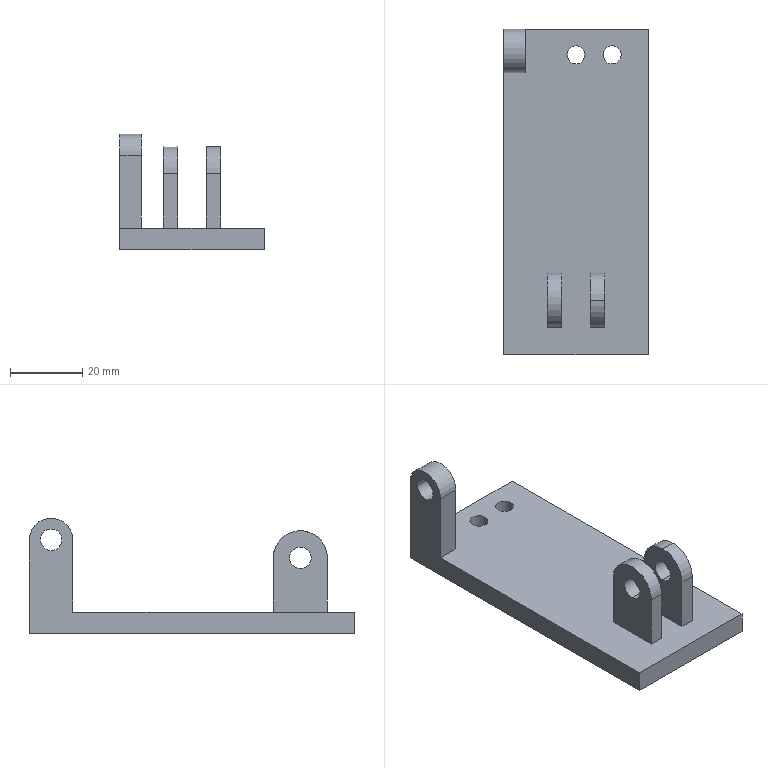Part | SolidWorks | features ICE 3, Extrusion 1, MirrorPattern 1 | 1 solid | 30 faces | box 40 x 90 x 32 mm | volume 25255 mm3 | plane 16 | cylinder 14 | commonest cylinder face diameters 6 x6 5 x4 15 x3 12 x1
STEP:
#1=CARTESIAN_POINT('',(-8.,-30.,24.));
#2=VERTEX_POINT('',#1);
#3=CARTESIAN_POINT('',(-8.,-30.,18.));
#4=VERTEX_POINT('',#3);
#5=CARTESIAN_POINT('',(-8.,-30.,21.));
#6=DIRECTION('',(1.,0.,0.));
#7=DIRECTION('',(0.,0.,-1.));
#8=AXIS2_PLACEMENT_3D('',#5,#6,#7);
#9=CIRCLE('',#8,3.);
#10=EDGE_CURVE('',#2,#4,#9,.T.);
#11=ORIENTED_EDGE('',*,*,#10,.F.);
#12=CARTESIAN_POINT('',(-4.,-30.,24.));
#13=VERTEX_POINT('',#12);
#14=CARTESIAN_POINT('',(-8.,-30.,24.));
#15=DIRECTION('',(1.,0.,0.));
#16=VECTOR('',#15,1000.);
#17=LINE('',#14,#16);
#18=EDGE_CURVE('',#2,#13,#17,.T.);
#19=ORIENTED_EDGE('',*,*,#18,.T.);
#20=CARTESIAN_POINT('',(-4.,-30.,18.));
#21=VERTEX_POINT('',#20);
#22=CARTESIAN_POINT('',(-4.,-30.,21.));
#23=DIRECTION('',(1.,0.,0.));
#24=DIRECTION('',(0.,0.,-1.));
#25=AXIS2_PLACEMENT_3D('',#22,#23,#24);
#26=CIRCLE('',#25,3.);
#27=EDGE_CURVE('',#13,#21,#26,.T.);
#28=ORIENTED_EDGE('',*,*,#27,.T.);
#29=CARTESIAN_POINT('',(-8.,-30.,18.));
#30=DIRECTION('',(1.,0.,0.));
#31=VECTOR('',#30,1000.);
#32=LINE('',#29,#31);
#33=EDGE_CURVE('',#4,#21,#32,.T.);
#34=ORIENTED_EDGE('',*,*,#33,.F.);
#35=EDGE_LOOP('',(#11,#19,#28,#34));
#36=FACE_OUTER_BOUND('',#35,.T.);
#37=CARTESIAN_POINT('',(-8.,-30.,21.));
#38=DIRECTION('',(1.,0.,0.));
#39=DIRECTION('',(0.,0.,-1.));
#40=AXIS2_PLACEMENT_3D('',#37,#38,#39);
#41=CYLINDRICAL_SURFACE('',#40,3.);
#42=ADVANCED_FACE('',(#36),#41,.F.);
#43=CARTESIAN_POINT('',(8.,-30.,24.));
#44=VERTEX_POINT('',#43);
#45=CARTESIAN_POINT('',(8.,-30.,18.));
#46=VERTEX_POINT('',#45);
#47=CARTESIAN_POINT('',(8.,-30.,21.));
#48=DIRECTION('',(1.,0.,0.));
#49=DIRECTION('',(0.,0.,-1.));
#50=AXIS2_PLACEMENT_3D('',#47,#48,#49);
#51=CIRCLE('',#50,3.);
#52=EDGE_CURVE('',#44,#46,#51,.T.);
#53=ORIENTED_EDGE('',*,*,#52,.T.);
#54=CARTESIAN_POINT('',(4.,-30.,18.));
#55=VERTEX_POINT('',#54);
#56=CARTESIAN_POINT('',(8.,-30.,18.));
#57=DIRECTION('',(-1.,0.,0.));
#58=VECTOR('',#57,1000.);
#59=LINE('',#56,#58);
#60=EDGE_CURVE('',#46,#55,#59,.T.);
#61=ORIENTED_EDGE('',*,*,#60,.T.);
#62=CARTESIAN_POINT('',(4.,-30.,24.));
#63=VERTEX_POINT('',#62);
#64=CARTESIAN_POINT('',(4.,-30.,21.));
#65=DIRECTION('',(1.,0.,0.));
#66=DIRECTION('',(0.,0.,-1.));
#67=AXIS2_PLACEMENT_3D('',#64,#65,#66);
#68=CIRCLE('',#67,3.);
#69=EDGE_CURVE('',#63,#55,#68,.T.);
#70=ORIENTED_EDGE('',*,*,#69,.F.);
#71=CARTESIAN_POINT('',(8.,-30.,24.));
#72=DIRECTION('',(-1.,0.,0.));
#73=VECTOR('',#72,1000.);
#74=LINE('',#71,#73);
#75=EDGE_CURVE('',#44,#63,#74,.T.);
#76=ORIENTED_EDGE('',*,*,#75,.F.);
#77=EDGE_LOOP('',(#53,#61,#70,#76));
#78=FACE_OUTER_BOUND('',#77,.T.);
#79=CARTESIAN_POINT('',(8.,-30.,21.));
#80=DIRECTION('',(-1.,0.,0.));
#81=DIRECTION('',(0.,0.,1.));
#82=AXIS2_PLACEMENT_3D('',#79,#80,#81);
#83=CYLINDRICAL_SURFACE('',#82,3.);
#84=ADVANCED_FACE('',(#78),#83,.F.);
#85=CARTESIAN_POINT('',(8.,-30.,28.5));
#86=VERTEX_POINT('',#85);
#87=CARTESIAN_POINT('',(8.,-37.5,21.));
#88=VERTEX_POINT('',#87);
#89=CARTESIAN_POINT('',(8.,-30.,21.));
#90=DIRECTION('',(1.,0.,0.));
#91=DIRECTION('',(0.,0.,-1.));
#92=AXIS2_PLACEMENT_3D('',#89,#90,#91);
#93=CIRCLE('',#92,7.5);
#94=EDGE_CURVE('',#86,#88,#93,.T.);
#95=ORIENTED_EDGE('',*,*,#94,.F.);
#96=CARTESIAN_POINT('',(4.,-30.,28.5));
#97=VERTEX_POINT('',#96);
#98=CARTESIAN_POINT('',(8.,-30.,28.5));
#99=DIRECTION('',(-1.,0.,0.));
#100=VECTOR('',#99,1000.);
#101=LINE('',#98,#100);
#102=EDGE_CURVE('',#86,#97,#101,.T.);
#103=ORIENTED_EDGE('',*,*,#102,.T.);
#104=CARTESIAN_POINT('',(4.,-37.5,21.));
#105=VERTEX_POINT('',#104);
#106=CARTESIAN_POINT('',(4.,-30.,21.));
#107=DIRECTION('',(1.,0.,0.));
#108=DIRECTION('',(0.,0.,-1.));
#109=AXIS2_PLACEMENT_3D('',#106,#107,#108);
#110=CIRCLE('',#109,7.5);
#111=EDGE_CURVE('',#97,#105,#110,.T.);
#112=ORIENTED_EDGE('',*,*,#111,.T.);
#113=CARTESIAN_POINT('',(8.,-37.5,21.));
#114=DIRECTION('',(-1.,0.,0.));
#115=VECTOR('',#114,1000.);
#116=LINE('',#113,#115);
#117=EDGE_CURVE('',#88,#105,#116,.T.);
#118=ORIENTED_EDGE('',*,*,#117,.F.);
#119=EDGE_LOOP('',(#95,#103,#112,#118));
#120=FACE_OUTER_BOUND('',#119,.T.);
#121=CARTESIAN_POINT('',(8.,-30.,21.));
#122=DIRECTION('',(-1.,0.,0.));
#123=DIRECTION('',(0.,0.,1.));
#124=AXIS2_PLACEMENT_3D('',#121,#122,#123);
#125=CYLINDRICAL_SURFACE('',#124,7.5);
#126=ADVANCED_FACE('',(#120),#125,.T.);
#127=CARTESIAN_POINT('',(-14.,42.,26.));
#128=VERTEX_POINT('',#127);
#129=CARTESIAN_POINT('',(-14.,36.,26.));
#130=VERTEX_POINT('',#129);
#131=CARTESIAN_POINT('',(-14.,39.,26.));
#132=DIRECTION('',(-1.,0.,0.));
#133=DIRECTION('',(0.,-1.,0.));
#134=AXIS2_PLACEMENT_3D('',#131,#132,#133);
#135=CIRCLE('',#134,3.);
#136=EDGE_CURVE('',#128,#130,#135,.T.);
#137=ORIENTED_EDGE('',*,*,#136,.F.);
#138=CARTESIAN_POINT('',(-20.,42.,26.));
#139=VERTEX_POINT('',#138);
#140=CARTESIAN_POINT('',(-14.,42.,26.));
#141=DIRECTION('',(-1.,0.,0.));
#142=VECTOR('',#141,1000.);
#143=LINE('',#140,#142);
#144=EDGE_CURVE('',#128,#139,#143,.T.);
#145=ORIENTED_EDGE('',*,*,#144,.T.);
#146=CARTESIAN_POINT('',(-20.,36.,26.));
#147=VERTEX_POINT('',#146);
#148=CARTESIAN_POINT('',(-20.,39.,26.));
#149=DIRECTION('',(-1.,0.,0.));
#150=DIRECTION('',(0.,-1.,0.));
#151=AXIS2_PLACEMENT_3D('',#148,#149,#150);
#152=CIRCLE('',#151,3.);
#153=EDGE_CURVE('',#139,#147,#152,.T.);
#154=ORIENTED_EDGE('',*,*,#153,.T.);
#155=CARTESIAN_POINT('',(-14.,36.,26.));
#156=DIRECTION('',(-1.,0.,0.));
#157=VECTOR('',#156,1000.);
#158=LINE('',#155,#157);
#159=EDGE_CURVE('',#130,#147,#158,.T.);
#160=ORIENTED_EDGE('',*,*,#159,.F.);
#161=EDGE_LOOP('',(#137,#145,#154,#160));
#162=FACE_OUTER_BOUND('',#161,.T.);
#163=CARTESIAN_POINT('',(-14.,39.,26.));
#164=DIRECTION('',(-1.,0.,0.));
#165=DIRECTION('',(0.,-1.,0.));
#166=AXIS2_PLACEMENT_3D('',#163,#164,#165);
#167=CYLINDRICAL_SURFACE('',#166,3.);
#168=ADVANCED_FACE('',(#162),#167,.F.);
#169=CARTESIAN_POINT('',(-2.5,38.,0.));
#170=VERTEX_POINT('',#169);
#171=CARTESIAN_POINT('',(2.5,38.,0.));
#172=VERTEX_POINT('',#171);
#173=CARTESIAN_POINT('',(0.,38.,0.));
#174=DIRECTION('',(0.,0.,1.));
#175=DIRECTION('',(1.,0.,0.));
#176=AXIS2_PLACEMENT_3D('',#173,#174,#175);
#177=CIRCLE('',#176,2.5);
#178=EDGE_CURVE('',#170,#172,#177,.T.);
#179=ORIENTED_EDGE('',*,*,#178,.F.);
#180=CARTESIAN_POINT('',(-2.5,38.,6.));
#181=VERTEX_POINT('',#180);
#182=CARTESIAN_POINT('',(-2.5,38.,0.));
#183=DIRECTION('',(0.,0.,1.));
#184=VECTOR('',#183,1000.);
#185=LINE('',#182,#184);
#186=EDGE_CURVE('',#170,#181,#185,.T.);
#187=ORIENTED_EDGE('',*,*,#186,.T.);
#188=CARTESIAN_POINT('',(2.5,38.,6.));
#189=VERTEX_POINT('',#188);
#190=CARTESIAN_POINT('',(0.,38.,6.));
#191=DIRECTION('',(0.,0.,1.));
#192=DIRECTION('',(1.,0.,0.));
#193=AXIS2_PLACEMENT_3D('',#190,#191,#192);
#194=CIRCLE('',#193,2.5);
#195=EDGE_CURVE('',#181,#189,#194,.T.);
#196=ORIENTED_EDGE('',*,*,#195,.T.);
#197=CARTESIAN_POINT('',(2.5,38.,0.));
#198=DIRECTION('',(0.,0.,1.));
#199=VECTOR('',#198,1000.);
#200=LINE('',#197,#199);
#201=EDGE_CURVE('',#172,#189,#200,.T.);
#202=ORIENTED_EDGE('',*,*,#201,.F.);
#203=EDGE_LOOP('',(#179,#187,#196,#202));
#204=FACE_OUTER_BOUND('',#203,.T.);
#205=CARTESIAN_POINT('',(0.,38.,0.));
#206=DIRECTION('',(0.,0.,1.));
#207=DIRECTION('',(1.,0.,0.));
#208=AXIS2_PLACEMENT_3D('',#205,#206,#207);
#209=CYLINDRICAL_SURFACE('',#208,2.5);
#210=ADVANCED_FACE('',(#204),#209,.F.);
#211=CARTESIAN_POINT('',(7.5,38.,0.));
#212=VERTEX_POINT('',#211);
#213=CARTESIAN_POINT('',(12.5,38.,0.));
#214=VERTEX_POINT('',#213);
#215=CARTESIAN_POINT('',(10.,38.,0.));
#216=DIRECTION('',(0.,0.,1.));
#217=DIRECTION('',(1.,0.,0.));
#218=AXIS2_PLACEMENT_3D('',#215,#216,#217);
#219=CIRCLE('',#218,2.5);
#220=EDGE_CURVE('',#212,#214,#219,.T.);
#221=ORIENTED_EDGE('',*,*,#220,.F.);
#222=CARTESIAN_POINT('',(7.5,38.,6.));
#223=VERTEX_POINT('',#222);
#224=CARTESIAN_POINT('',(7.5,38.,0.));
#225=DIRECTION('',(0.,0.,1.));
#226=VECTOR('',#225,1000.);
#227=LINE('',#224,#226);
#228=EDGE_CURVE('',#212,#223,#227,.T.);
#229=ORIENTED_EDGE('',*,*,#228,.T.);
#230=CARTESIAN_POINT('',(12.5,38.,6.));
#231=VERTEX_POINT('',#230);
#232=CARTESIAN_POINT('',(10.,38.,6.));
#233=DIRECTION('',(0.,0.,1.));
#234=DIRECTION('',(1.,0.,0.));
#235=AXIS2_PLACEMENT_3D('',#232,#233,#234);
#236=CIRCLE('',#235,2.5);
#237=EDGE_CURVE('',#223,#231,#236,.T.);
#238=ORIENTED_EDGE('',*,*,#237,.T.);
#239=CARTESIAN_POINT('',(12.5,38.,0.));
#240=DIRECTION('',(0.,0.,1.));
#241=VECTOR('',#240,1000.);
#242=LINE('',#239,#241);
#243=EDGE_CURVE('',#214,#231,#242,.T.);
#244=ORIENTED_EDGE('',*,*,#243,.F.);
#245=EDGE_LOOP('',(#221,#229,#238,#244));
#246=FACE_OUTER_BOUND('',#245,.T.);
#247=CARTESIAN_POINT('',(10.,38.,0.));
#248=DIRECTION('',(0.,0.,1.));
#249=DIRECTION('',(1.,0.,0.));
#250=AXIS2_PLACEMENT_3D('',#247,#248,#249);
#251=CYLINDRICAL_SURFACE('',#250,2.5);
#252=ADVANCED_FACE('',(#246),#251,.F.);
#253=CARTESIAN_POINT('',(-8.,-37.5,6.));
#254=VERTEX_POINT('',#253);
#255=CARTESIAN_POINT('',(-8.,-22.5,6.));
#256=VERTEX_POINT('',#255);
#257=CARTESIAN_POINT('',(-8.,-22.5,6.));
#258=DIRECTION('',(0.,1.,0.));
#259=VECTOR('',#258,1000.);
#260=LINE('',#257,#259);
#261=EDGE_CURVE('',#254,#256,#260,.T.);
#262=ORIENTED_EDGE('',*,*,#261,.T.);
#263=CARTESIAN_POINT('',(-4.,-22.5,6.));
#264=VERTEX_POINT('',#263);
#265=CARTESIAN_POINT('',(-8.,-22.5,6.));
#266=DIRECTION('',(1.,0.,0.));
#267=VECTOR('',#266,1000.);
#268=LINE('',#265,#267);
#269=EDGE_CURVE('',#256,#264,#268,.T.);
#270=ORIENTED_EDGE('',*,*,#269,.T.);
#271=CARTESIAN_POINT('',(-4.,-37.5,6.));
#272=VERTEX_POINT('',#271);
#273=CARTESIAN_POINT('',(-4.,-22.5,6.));
#274=DIRECTION('',(0.,1.,0.));
#275=VECTOR('',#274,1000.);
#276=LINE('',#273,#275);
#277=EDGE_CURVE('',#272,#264,#276,.T.);
#278=ORIENTED_EDGE('',*,*,#277,.F.);
#279=CARTESIAN_POINT('',(-8.,-37.5,6.));
#280=DIRECTION('',(1.,0.,0.));
#281=VECTOR('',#280,1000.);
#282=LINE('',#279,#281);
#283=EDGE_CURVE('',#254,#272,#282,.T.);
#284=ORIENTED_EDGE('',*,*,#283,.F.);
#285=EDGE_LOOP('',(#262,#270,#278,#284));
#286=FACE_BOUND('',#285,.T.);
#287=CARTESIAN_POINT('',(0.,38.,6.));
#288=DIRECTION('',(0.,0.,1.));
#289=DIRECTION('',(1.,0.,0.));
#290=AXIS2_PLACEMENT_3D('',#287,#288,#289);
#291=CIRCLE('',#290,2.5);
#292=EDGE_CURVE('',#189,#181,#291,.T.);
#293=ORIENTED_EDGE('',*,*,#292,.F.);
#294=ORIENTED_EDGE('',*,*,#195,.F.);
#295=EDGE_LOOP('',(#293,#294));
#296=FACE_BOUND('',#295,.T.);
#297=CARTESIAN_POINT('',(10.,38.,6.));
#298=DIRECTION('',(0.,0.,1.));
#299=DIRECTION('',(1.,0.,0.));
#300=AXIS2_PLACEMENT_3D('',#297,#298,#299);
#301=CIRCLE('',#300,2.5);
#302=EDGE_CURVE('',#231,#223,#301,.T.);
#303=ORIENTED_EDGE('',*,*,#302,.F.);
#304=ORIENTED_EDGE('',*,*,#237,.F.);
#305=EDGE_LOOP('',(#303,#304));
#306=FACE_BOUND('',#305,.T.);
#307=CARTESIAN_POINT('',(20.,45.,6.));
#308=VERTEX_POINT('',#307);
#309=CARTESIAN_POINT('',(-14.,45.,6.));
#310=VERTEX_POINT('',#309);
#311=CARTESIAN_POINT('',(-20.,45.,6.));
#312=DIRECTION('',(-1.,0.,0.));
#313=VECTOR('',#312,1000.);
#314=LINE('',#311,#313);
#315=EDGE_CURVE('',#308,#310,#314,.T.);
#316=ORIENTED_EDGE('',*,*,#315,.T.);
#317=CARTESIAN_POINT('',(-14.,33.,6.));
#318=VERTEX_POINT('',#317);
#319=CARTESIAN_POINT('',(-14.,45.,6.));
#320=DIRECTION('',(0.,-1.,0.));
#321=VECTOR('',#320,1000.);
#322=LINE('',#319,#321);
#323=EDGE_CURVE('',#310,#318,#322,.T.);
#324=ORIENTED_EDGE('',*,*,#323,.T.);
#325=CARTESIAN_POINT('',(-20.,33.,6.));
#326=VERTEX_POINT('',#325);
#327=CARTESIAN_POINT('',(-14.,33.,6.));
#328=DIRECTION('',(-1.,0.,0.));
#329=VECTOR('',#328,1000.);
#330=LINE('',#327,#329);
#331=EDGE_CURVE('',#318,#326,#330,.T.);
#332=ORIENTED_EDGE('',*,*,#331,.T.);
#333=CARTESIAN_POINT('',(-20.,-45.,6.));
#334=VERTEX_POINT('',#333);
#335=CARTESIAN_POINT('',(-20.,45.,6.));
#336=DIRECTION('',(0.,-1.,0.));
#337=VECTOR('',#336,1000.);
#338=LINE('',#335,#337);
#339=EDGE_CURVE('',#326,#334,#338,.T.);
#340=ORIENTED_EDGE('',*,*,#339,.T.);
#341=CARTESIAN_POINT('',(20.,-45.,6.));
#342=VERTEX_POINT('',#341);
#343=CARTESIAN_POINT('',(-20.,-45.,6.));
#344=DIRECTION('',(1.,0.,0.));
#345=VECTOR('',#344,1000.);
#346=LINE('',#343,#345);
#347=EDGE_CURVE('',#334,#342,#346,.T.);
#348=ORIENTED_EDGE('',*,*,#347,.T.);
#349=CARTESIAN_POINT('',(20.,45.,6.));
#350=DIRECTION('',(0.,1.,0.));
#351=VECTOR('',#350,1000.);
#352=LINE('',#349,#351);
#353=EDGE_CURVE('',#342,#308,#352,.T.);
#354=ORIENTED_EDGE('',*,*,#353,.T.);
#355=EDGE_LOOP('',(#316,#324,#332,#340,#348,#354));
#356=FACE_OUTER_BOUND('',#355,.T.);
#357=CARTESIAN_POINT('',(8.,-37.5,6.));
#358=VERTEX_POINT('',#357);
#359=CARTESIAN_POINT('',(8.,-22.5,6.));
#360=VERTEX_POINT('',#359);
#361=CARTESIAN_POINT('',(8.,-22.5,6.));
#362=DIRECTION('',(0.,1.,0.));
#363=VECTOR('',#362,1000.);
#364=LINE('',#361,#363);
#365=EDGE_CURVE('',#358,#360,#364,.T.);
#366=ORIENTED_EDGE('',*,*,#365,.F.);
#367=CARTESIAN_POINT('',(4.,-37.5,6.));
#368=VERTEX_POINT('',#367);
#369=CARTESIAN_POINT('',(8.,-37.5,6.));
#370=DIRECTION('',(-1.,0.,0.));
#371=VECTOR('',#370,1000.);
#372=LINE('',#369,#371);
#373=EDGE_CURVE('',#358,#368,#372,.T.);
#374=ORIENTED_EDGE('',*,*,#373,.T.);
#375=CARTESIAN_POINT('',(4.,-22.5,6.));
#376=VERTEX_POINT('',#375);
#377=CARTESIAN_POINT('',(4.,-22.5,6.));
#378=DIRECTION('',(0.,1.,0.));
#379=VECTOR('',#378,1000.);
#380=LINE('',#377,#379);
#381=EDGE_CURVE('',#368,#376,#380,.T.);
#382=ORIENTED_EDGE('',*,*,#381,.T.);
#383=CARTESIAN_POINT('',(8.,-22.5,6.));
#384=DIRECTION('',(-1.,0.,0.));
#385=VECTOR('',#384,1000.);
#386=LINE('',#383,#385);
#387=EDGE_CURVE('',#360,#376,#386,.T.);
#388=ORIENTED_EDGE('',*,*,#387,.F.);
#389=EDGE_LOOP('',(#366,#374,#382,#388));
#390=FACE_BOUND('',#389,.T.);
#391=CARTESIAN_POINT('',(0.,0.,6.));
#392=DIRECTION('',(0.,0.,1.));
#393=DIRECTION('',(1.,0.,0.));
#394=AXIS2_PLACEMENT_3D('',#391,#392,#393);
#395=PLANE('',#394);
#396=ADVANCED_FACE('',(#286,#296,#306,#356,#390),#395,.T.);
#397=CARTESIAN_POINT('',(20.,-45.,0.));
#398=VERTEX_POINT('',#397);
#399=CARTESIAN_POINT('',(20.,45.,0.));
#400=VERTEX_POINT('',#399);
#401=CARTESIAN_POINT('',(20.,45.,0.));
#402=DIRECTION('',(0.,1.,0.));
#403=VECTOR('',#402,1000.);
#404=LINE('',#401,#403);
#405=EDGE_CURVE('',#398,#400,#404,.T.);
#406=ORIENTED_EDGE('',*,*,#405,.T.);
#407=CARTESIAN_POINT('',(20.,45.,6.));
#408=DIRECTION('',(0.,0.,-1.));
#409=VECTOR('',#408,1000.);
#410=LINE('',#407,#409);
#411=EDGE_CURVE('',#308,#400,#410,.T.);
#412=ORIENTED_EDGE('',*,*,#411,.F.);
#413=ORIENTED_EDGE('',*,*,#353,.F.);
#414=CARTESIAN_POINT('',(20.,-45.,6.));
#415=DIRECTION('',(0.,0.,-1.));
#416=VECTOR('',#415,1000.);
#417=LINE('',#414,#416);
#418=EDGE_CURVE('',#342,#398,#417,.T.);
#419=ORIENTED_EDGE('',*,*,#418,.T.);
#420=EDGE_LOOP('',(#406,#412,#413,#419));
#421=FACE_OUTER_BOUND('',#420,.T.);
#422=CARTESIAN_POINT('',(20.,45.,6.));
#423=DIRECTION('',(-1.,0.,0.));
#424=DIRECTION('',(0.,-1.,0.));
#425=AXIS2_PLACEMENT_3D('',#422,#423,#424);
#426=PLANE('',#425);
#427=ADVANCED_FACE('',(#421),#426,.F.);
#428=CARTESIAN_POINT('',(-20.,45.,0.));
#429=VERTEX_POINT('',#428);
#430=CARTESIAN_POINT('',(-20.,45.,0.));
#431=DIRECTION('',(-1.,0.,0.));
#432=VECTOR('',#431,1000.);
#433=LINE('',#430,#432);
#434=EDGE_CURVE('',#400,#429,#433,.T.);
#435=ORIENTED_EDGE('',*,*,#434,.T.);
#436=CARTESIAN_POINT('',(-20.,45.,26.));
#437=VERTEX_POINT('',#436);
#438=CARTESIAN_POINT('',(-20.,45.,6.));
#439=DIRECTION('',(0.,0.,-1.));
#440=VECTOR('',#439,1000.);
#441=LINE('',#438,#440);
#442=EDGE_CURVE('',#437,#429,#441,.T.);
#443=ORIENTED_EDGE('',*,*,#442,.F.);
#444=CARTESIAN_POINT('',(-14.,45.,26.));
#445=VERTEX_POINT('',#444);
#446=CARTESIAN_POINT('',(-14.,45.,26.));
#447=DIRECTION('',(-1.,0.,0.));
#448=VECTOR('',#447,1000.);
#449=LINE('',#446,#448);
#450=EDGE_CURVE('',#445,#437,#449,.T.);
#451=ORIENTED_EDGE('',*,*,#450,.F.);
#452=CARTESIAN_POINT('',(-14.,45.,26.));
#453=DIRECTION('',(0.,0.,-1.));
#454=VECTOR('',#453,1000.);
#455=LINE('',#452,#454);
#456=EDGE_CURVE('',#445,#310,#455,.T.);
#457=ORIENTED_EDGE('',*,*,#456,.T.);
#458=ORIENTED_EDGE('',*,*,#315,.F.);
#459=ORIENTED_EDGE('',*,*,#411,.T.);
#460=EDGE_LOOP('',(#435,#443,#451,#457,#458,#459));
#461=FACE_OUTER_BOUND('',#460,.T.);
#462=CARTESIAN_POINT('',(-20.,45.,6.));
#463=DIRECTION('',(0.,-1.,0.));
#464=DIRECTION('',(0.,0.,-1.));
#465=AXIS2_PLACEMENT_3D('',#462,#463,#464);
#466=PLANE('',#465);
#467=ADVANCED_FACE('',(#461),#466,.F.);
#468=CARTESIAN_POINT('',(-20.,-45.,0.));
#469=VERTEX_POINT('',#468);
#470=CARTESIAN_POINT('',(-20.,45.,0.));
#471=DIRECTION('',(0.,-1.,0.));
#472=VECTOR('',#471,1000.);
#473=LINE('',#470,#472);
#474=EDGE_CURVE('',#429,#469,#473,.T.);
#475=ORIENTED_EDGE('',*,*,#474,.T.);
#476=CARTESIAN_POINT('',(-20.,-45.,6.));
#477=DIRECTION('',(0.,0.,-1.));
#478=VECTOR('',#477,1000.);
#479=LINE('',#476,#478);
#480=EDGE_CURVE('',#334,#469,#479,.T.);
#481=ORIENTED_EDGE('',*,*,#480,.F.);
#482=ORIENTED_EDGE('',*,*,#339,.F.);
#483=CARTESIAN_POINT('',(-20.,33.,26.));
#484=VERTEX_POINT('',#483);
#485=CARTESIAN_POINT('',(-20.,33.,6.));
#486=DIRECTION('',(0.,0.,1.));
#487=VECTOR('',#486,1000.);
#488=LINE('',#485,#487);
#489=EDGE_CURVE('',#326,#484,#488,.T.);
#490=ORIENTED_EDGE('',*,*,#489,.T.);
#491=CARTESIAN_POINT('',(-20.,39.,26.));
#492=DIRECTION('',(-1.,0.,0.));
#493=DIRECTION('',(0.,-1.,0.));
#494=AXIS2_PLACEMENT_3D('',#491,#492,#493);
#495=CIRCLE('',#494,6.);
#496=EDGE_CURVE('',#484,#437,#495,.T.);
#497=ORIENTED_EDGE('',*,*,#496,.T.);
#498=ORIENTED_EDGE('',*,*,#442,.T.);
#499=EDGE_LOOP('',(#475,#481,#482,#490,#497,#498));
#500=FACE_OUTER_BOUND('',#499,.T.);
#501=CARTESIAN_POINT('',(-20.,39.,26.));
#502=DIRECTION('',(-1.,0.,0.));
#503=DIRECTION('',(0.,-1.,0.));
#504=AXIS2_PLACEMENT_3D('',#501,#502,#503);
#505=CIRCLE('',#504,3.);
#506=EDGE_CURVE('',#147,#139,#505,.T.);
#507=ORIENTED_EDGE('',*,*,#506,.F.);
#508=ORIENTED_EDGE('',*,*,#153,.F.);
#509=EDGE_LOOP('',(#507,#508));
#510=FACE_BOUND('',#509,.T.);
#511=CARTESIAN_POINT('',(-20.,45.,6.));
#512=DIRECTION('',(1.,0.,0.));
#513=DIRECTION('',(0.,1.,0.));
#514=AXIS2_PLACEMENT_3D('',#511,#512,#513);
#515=PLANE('',#514);
#516=ADVANCED_FACE('',(#500,#510),#515,.F.);
#517=CARTESIAN_POINT('',(-20.,-45.,0.));
#518=DIRECTION('',(1.,0.,0.));
#519=VECTOR('',#518,1000.);
#520=LINE('',#517,#519);
#521=EDGE_CURVE('',#469,#398,#520,.T.);
#522=ORIENTED_EDGE('',*,*,#521,.T.);
#523=ORIENTED_EDGE('',*,*,#418,.F.);
#524=ORIENTED_EDGE('',*,*,#347,.F.);
#525=ORIENTED_EDGE('',*,*,#480,.T.);
#526=EDGE_LOOP('',(#522,#523,#524,#525));
#527=FACE_OUTER_BOUND('',#526,.T.);
#528=CARTESIAN_POINT('',(-20.,-45.,6.));
#529=DIRECTION('',(0.,1.,0.));
#530=DIRECTION('',(0.,0.,1.));
#531=AXIS2_PLACEMENT_3D('',#528,#529,#530);
#532=PLANE('',#531);
#533=ADVANCED_FACE('',(#527),#532,.F.);
#534=CARTESIAN_POINT('',(0.,38.,0.));
#535=DIRECTION('',(0.,0.,1.));
#536=DIRECTION('',(1.,0.,0.));
#537=AXIS2_PLACEMENT_3D('',#534,#535,#536);
#538=CIRCLE('',#537,2.5);
#539=EDGE_CURVE('',#172,#170,#538,.T.);
#540=ORIENTED_EDGE('',*,*,#539,.T.);
#541=ORIENTED_EDGE('',*,*,#178,.T.);
#542=EDGE_LOOP('',(#540,#541));
#543=FACE_BOUND('',#542,.T.);
#544=CARTESIAN_POINT('',(10.,38.,0.));
#545=DIRECTION('',(0.,0.,1.));
#546=DIRECTION('',(1.,0.,0.));
#547=AXIS2_PLACEMENT_3D('',#544,#545,#546);
#548=CIRCLE('',#547,2.5);
#549=EDGE_CURVE('',#214,#212,#548,.T.);
#550=ORIENTED_EDGE('',*,*,#549,.T.);
#551=ORIENTED_EDGE('',*,*,#220,.T.);
#552=EDGE_LOOP('',(#550,#551));
#553=FACE_BOUND('',#552,.T.);
#554=ORIENTED_EDGE('',*,*,#405,.F.);
#555=ORIENTED_EDGE('',*,*,#521,.F.);
#556=ORIENTED_EDGE('',*,*,#474,.F.);
#557=ORIENTED_EDGE('',*,*,#434,.F.);
#558=EDGE_LOOP('',(#554,#555,#556,#557));
#559=FACE_OUTER_BOUND('',#558,.T.);
#560=CARTESIAN_POINT('',(0.,0.,0.));
#561=DIRECTION('',(0.,0.,1.));
#562=DIRECTION('',(1.,0.,0.));
#563=AXIS2_PLACEMENT_3D('',#560,#561,#562);
#564=PLANE('',#563);
#565=ADVANCED_FACE('',(#543,#553,#559),#564,.F.);
#566=ORIENTED_EDGE('',*,*,#228,.F.);
#567=ORIENTED_EDGE('',*,*,#549,.F.);
#568=ORIENTED_EDGE('',*,*,#243,.T.);
#569=ORIENTED_EDGE('',*,*,#302,.T.);
#570=EDGE_LOOP('',(#566,#567,#568,#569));
#571=FACE_OUTER_BOUND('',#570,.T.);
#572=CARTESIAN_POINT('',(10.,38.,0.));
#573=DIRECTION('',(0.,0.,1.));
#574=DIRECTION('',(1.,0.,0.));
#575=AXIS2_PLACEMENT_3D('',#572,#573,#574);
#576=CYLINDRICAL_SURFACE('',#575,2.5);
#577=ADVANCED_FACE('',(#571),#576,.F.);
#578=ORIENTED_EDGE('',*,*,#186,.F.);
#579=ORIENTED_EDGE('',*,*,#539,.F.);
#580=ORIENTED_EDGE('',*,*,#201,.T.);
#581=ORIENTED_EDGE('',*,*,#292,.T.);
#582=EDGE_LOOP('',(#578,#579,#580,#581));
#583=FACE_OUTER_BOUND('',#582,.T.);
#584=CARTESIAN_POINT('',(0.,38.,0.));
#585=DIRECTION('',(0.,0.,1.));
#586=DIRECTION('',(1.,0.,0.));
#587=AXIS2_PLACEMENT_3D('',#584,#585,#586);
#588=CYLINDRICAL_SURFACE('',#587,2.5);
#589=ADVANCED_FACE('',(#583),#588,.F.);
#590=ORIENTED_EDGE('',*,*,#496,.F.);
#591=CARTESIAN_POINT('',(-14.,33.,26.));
#592=VERTEX_POINT('',#591);
#593=CARTESIAN_POINT('',(-14.,33.,26.));
#594=DIRECTION('',(-1.,0.,0.));
#595=VECTOR('',#594,1000.);
#596=LINE('',#593,#595);
#597=EDGE_CURVE('',#592,#484,#596,.T.);
#598=ORIENTED_EDGE('',*,*,#597,.F.);
#599=CARTESIAN_POINT('',(-14.,39.,26.));
#600=DIRECTION('',(-1.,0.,0.));
#601=DIRECTION('',(0.,-1.,0.));
#602=AXIS2_PLACEMENT_3D('',#599,#600,#601);
#603=CIRCLE('',#602,6.);
#604=EDGE_CURVE('',#592,#445,#603,.T.);
#605=ORIENTED_EDGE('',*,*,#604,.T.);
#606=ORIENTED_EDGE('',*,*,#450,.T.);
#607=EDGE_LOOP('',(#590,#598,#605,#606));
#608=FACE_OUTER_BOUND('',#607,.T.);
#609=CARTESIAN_POINT('',(-14.,39.,26.));
#610=DIRECTION('',(-1.,0.,0.));
#611=DIRECTION('',(0.,-1.,0.));
#612=AXIS2_PLACEMENT_3D('',#609,#610,#611);
#613=CYLINDRICAL_SURFACE('',#612,6.);
#614=ADVANCED_FACE('',(#608),#613,.T.);
#615=ORIENTED_EDGE('',*,*,#489,.F.);
#616=ORIENTED_EDGE('',*,*,#331,.F.);
#617=CARTESIAN_POINT('',(-14.,33.,6.));
#618=DIRECTION('',(0.,0.,1.));
#619=VECTOR('',#618,1000.);
#620=LINE('',#617,#619);
#621=EDGE_CURVE('',#318,#592,#620,.T.);
#622=ORIENTED_EDGE('',*,*,#621,.T.);
#623=ORIENTED_EDGE('',*,*,#597,.T.);
#624=EDGE_LOOP('',(#615,#616,#622,#623));
#625=FACE_OUTER_BOUND('',#624,.T.);
#626=CARTESIAN_POINT('',(-14.,33.,6.));
#627=DIRECTION('',(0.,-1.,0.));
#628=DIRECTION('',(1.,0.,0.));
#629=AXIS2_PLACEMENT_3D('',#626,#627,#628);
#630=PLANE('',#629);
#631=ADVANCED_FACE('',(#625),#630,.T.);
#632=CARTESIAN_POINT('',(-14.,39.,26.));
#633=DIRECTION('',(-1.,0.,0.));
#634=DIRECTION('',(0.,-1.,0.));
#635=AXIS2_PLACEMENT_3D('',#632,#633,#634);
#636=CIRCLE('',#635,3.);
#637=EDGE_CURVE('',#130,#128,#636,.T.);
#638=ORIENTED_EDGE('',*,*,#637,.T.);
#639=ORIENTED_EDGE('',*,*,#136,.T.);
#640=EDGE_LOOP('',(#638,#639));
#641=FACE_BOUND('',#640,.T.);
#642=ORIENTED_EDGE('',*,*,#604,.F.);
#643=ORIENTED_EDGE('',*,*,#621,.F.);
#644=ORIENTED_EDGE('',*,*,#323,.F.);
#645=ORIENTED_EDGE('',*,*,#456,.F.);
#646=EDGE_LOOP('',(#642,#643,#644,#645));
#647=FACE_OUTER_BOUND('',#646,.T.);
#648=CARTESIAN_POINT('',(-14.,39.,26.));
#649=DIRECTION('',(-1.,0.,0.));
#650=DIRECTION('',(0.,-1.,0.));
#651=AXIS2_PLACEMENT_3D('',#648,#649,#650);
#652=PLANE('',#651);
#653=ADVANCED_FACE('',(#641,#647),#652,.F.);
#654=ORIENTED_EDGE('',*,*,#144,.F.);
#655=ORIENTED_EDGE('',*,*,#637,.F.);
#656=ORIENTED_EDGE('',*,*,#159,.T.);
#657=ORIENTED_EDGE('',*,*,#506,.T.);
#658=EDGE_LOOP('',(#654,#655,#656,#657));
#659=FACE_OUTER_BOUND('',#658,.T.);
#660=CARTESIAN_POINT('',(-14.,39.,26.));
#661=DIRECTION('',(-1.,0.,0.));
#662=DIRECTION('',(0.,-1.,0.));
#663=AXIS2_PLACEMENT_3D('',#660,#661,#662);
#664=CYLINDRICAL_SURFACE('',#663,3.);
#665=ADVANCED_FACE('',(#659),#664,.F.);
#666=CARTESIAN_POINT('',(8.,-22.5,21.));
#667=VERTEX_POINT('',#666);
#668=CARTESIAN_POINT('',(8.,-30.,21.));
#669=DIRECTION('',(1.,0.,0.));
#670=DIRECTION('',(0.,0.,-1.));
#671=AXIS2_PLACEMENT_3D('',#668,#669,#670);
#672=CIRCLE('',#671,7.5);
#673=EDGE_CURVE('',#667,#86,#672,.T.);
#674=ORIENTED_EDGE('',*,*,#673,.T.);
#675=ORIENTED_EDGE('',*,*,#94,.T.);
#676=CARTESIAN_POINT('',(8.,-37.5,6.));
#677=DIRECTION('',(0.,0.,-1.));
#678=VECTOR('',#677,1000.);
#679=LINE('',#676,#678);
#680=EDGE_CURVE('',#88,#358,#679,.T.);
#681=ORIENTED_EDGE('',*,*,#680,.T.);
#682=ORIENTED_EDGE('',*,*,#365,.T.);
#683=CARTESIAN_POINT('',(8.,-22.5,21.));
#684=DIRECTION('',(0.,0.,1.));
#685=VECTOR('',#684,1000.);
#686=LINE('',#683,#685);
#687=EDGE_CURVE('',#360,#667,#686,.T.);
#688=ORIENTED_EDGE('',*,*,#687,.T.);
#689=EDGE_LOOP('',(#674,#675,#681,#682,#688));
#690=FACE_OUTER_BOUND('',#689,.T.);
#691=ORIENTED_EDGE('',*,*,#52,.F.);
#692=CARTESIAN_POINT('',(8.,-30.,21.));
#693=DIRECTION('',(1.,0.,0.));
#694=DIRECTION('',(0.,0.,-1.));
#695=AXIS2_PLACEMENT_3D('',#692,#693,#694);
#696=CIRCLE('',#695,3.);
#697=EDGE_CURVE('',#46,#44,#696,.T.);
#698=ORIENTED_EDGE('',*,*,#697,.F.);
#699=EDGE_LOOP('',(#691,#698));
#700=FACE_BOUND('',#699,.T.);
#701=CARTESIAN_POINT('',(8.,-30.,21.));
#702=DIRECTION('',(1.,0.,0.));
#703=DIRECTION('',(0.,0.,-1.));
#704=AXIS2_PLACEMENT_3D('',#701,#702,#703);
#705=PLANE('',#704);
#706=ADVANCED_FACE('',(#690,#700),#705,.T.);
#707=CARTESIAN_POINT('',(4.,-22.5,21.));
#708=VERTEX_POINT('',#707);
#709=CARTESIAN_POINT('',(4.,-30.,21.));
#710=DIRECTION('',(1.,0.,0.));
#711=DIRECTION('',(0.,0.,-1.));
#712=AXIS2_PLACEMENT_3D('',#709,#710,#711);
#713=CIRCLE('',#712,7.5);
#714=EDGE_CURVE('',#708,#97,#713,.T.);
#715=ORIENTED_EDGE('',*,*,#714,.F.);
#716=CARTESIAN_POINT('',(4.,-22.5,21.));
#717=DIRECTION('',(0.,0.,1.));
#718=VECTOR('',#717,1000.);
#719=LINE('',#716,#718);
#720=EDGE_CURVE('',#376,#708,#719,.T.);
#721=ORIENTED_EDGE('',*,*,#720,.F.);
#722=ORIENTED_EDGE('',*,*,#381,.F.);
#723=CARTESIAN_POINT('',(4.,-37.5,6.));
#724=DIRECTION('',(0.,0.,-1.));
#725=VECTOR('',#724,1000.);
#726=LINE('',#723,#725);
#727=EDGE_CURVE('',#105,#368,#726,.T.);
#728=ORIENTED_EDGE('',*,*,#727,.F.);
#729=ORIENTED_EDGE('',*,*,#111,.F.);
#730=EDGE_LOOP('',(#715,#721,#722,#728,#729));
#731=FACE_OUTER_BOUND('',#730,.T.);
#732=ORIENTED_EDGE('',*,*,#69,.T.);
#733=CARTESIAN_POINT('',(4.,-30.,21.));
#734=DIRECTION('',(1.,0.,0.));
#735=DIRECTION('',(0.,0.,-1.));
#736=AXIS2_PLACEMENT_3D('',#733,#734,#735);
#737=CIRCLE('',#736,3.);
#738=EDGE_CURVE('',#55,#63,#737,.T.);
#739=ORIENTED_EDGE('',*,*,#738,.T.);
#740=EDGE_LOOP('',(#732,#739));
#741=FACE_BOUND('',#740,.T.);
#742=CARTESIAN_POINT('',(4.,-30.,21.));
#743=DIRECTION('',(1.,0.,0.));
#744=DIRECTION('',(0.,0.,-1.));
#745=AXIS2_PLACEMENT_3D('',#742,#743,#744);
#746=PLANE('',#745);
#747=ADVANCED_FACE('',(#731,#741),#746,.F.);
#748=ORIENTED_EDGE('',*,*,#102,.F.);
#749=ORIENTED_EDGE('',*,*,#673,.F.);
#750=CARTESIAN_POINT('',(8.,-22.5,21.));
#751=DIRECTION('',(-1.,0.,0.));
#752=VECTOR('',#751,1000.);
#753=LINE('',#750,#752);
#754=EDGE_CURVE('',#667,#708,#753,.T.);
#755=ORIENTED_EDGE('',*,*,#754,.T.);
#756=ORIENTED_EDGE('',*,*,#714,.T.);
#757=EDGE_LOOP('',(#748,#749,#755,#756));
#758=FACE_OUTER_BOUND('',#757,.T.);
#759=CARTESIAN_POINT('',(8.,-30.,21.));
#760=DIRECTION('',(-1.,0.,0.));
#761=DIRECTION('',(0.,0.,1.));
#762=AXIS2_PLACEMENT_3D('',#759,#760,#761);
#763=CYLINDRICAL_SURFACE('',#762,7.5);
#764=ADVANCED_FACE('',(#758),#763,.T.);
#765=ORIENTED_EDGE('',*,*,#727,.T.);
#766=ORIENTED_EDGE('',*,*,#373,.F.);
#767=ORIENTED_EDGE('',*,*,#680,.F.);
#768=ORIENTED_EDGE('',*,*,#117,.T.);
#769=EDGE_LOOP('',(#765,#766,#767,#768));
#770=FACE_OUTER_BOUND('',#769,.T.);
#771=CARTESIAN_POINT('',(8.,-37.5,6.));
#772=DIRECTION('',(0.,1.,0.));
#773=DIRECTION('',(0.,0.,1.));
#774=AXIS2_PLACEMENT_3D('',#771,#772,#773);
#775=PLANE('',#774);
#776=ADVANCED_FACE('',(#770),#775,.F.);
#777=ORIENTED_EDGE('',*,*,#720,.T.);
#778=ORIENTED_EDGE('',*,*,#754,.F.);
#779=ORIENTED_EDGE('',*,*,#687,.F.);
#780=ORIENTED_EDGE('',*,*,#387,.T.);
#781=EDGE_LOOP('',(#777,#778,#779,#780));
#782=FACE_OUTER_BOUND('',#781,.T.);
#783=CARTESIAN_POINT('',(8.,-22.5,21.));
#784=DIRECTION('',(0.,-1.,0.));
#785=DIRECTION('',(0.,0.,-1.));
#786=AXIS2_PLACEMENT_3D('',#783,#784,#785);
#787=PLANE('',#786);
#788=ADVANCED_FACE('',(#782),#787,.F.);
#789=ORIENTED_EDGE('',*,*,#60,.F.);
#790=ORIENTED_EDGE('',*,*,#697,.T.);
#791=ORIENTED_EDGE('',*,*,#75,.T.);
#792=ORIENTED_EDGE('',*,*,#738,.F.);
#793=EDGE_LOOP('',(#789,#790,#791,#792));
#794=FACE_OUTER_BOUND('',#793,.T.);
#795=CARTESIAN_POINT('',(8.,-30.,21.));
#796=DIRECTION('',(-1.,0.,0.));
#797=DIRECTION('',(0.,0.,1.));
#798=AXIS2_PLACEMENT_3D('',#795,#796,#797);
#799=CYLINDRICAL_SURFACE('',#798,3.);
#800=ADVANCED_FACE('',(#794),#799,.F.);
#801=CARTESIAN_POINT('',(-4.,-22.5,21.));
#802=VERTEX_POINT('',#801);
#803=CARTESIAN_POINT('',(-4.,-37.5,21.));
#804=VERTEX_POINT('',#803);
#805=CARTESIAN_POINT('',(-4.,-30.,21.));
#806=DIRECTION('',(1.,0.,0.));
#807=DIRECTION('',(0.,0.,-1.));
#808=AXIS2_PLACEMENT_3D('',#805,#806,#807);
#809=CIRCLE('',#808,7.5);
#810=EDGE_CURVE('',#802,#804,#809,.T.);
#811=ORIENTED_EDGE('',*,*,#810,.F.);
#812=CARTESIAN_POINT('',(-8.,-22.5,21.));
#813=VERTEX_POINT('',#812);
#814=CARTESIAN_POINT('',(-8.,-22.5,21.));
#815=DIRECTION('',(1.,0.,0.));
#816=VECTOR('',#815,1000.);
#817=LINE('',#814,#816);
#818=EDGE_CURVE('',#813,#802,#817,.T.);
#819=ORIENTED_EDGE('',*,*,#818,.F.);
#820=CARTESIAN_POINT('',(-8.,-37.5,21.));
#821=VERTEX_POINT('',#820);
#822=CARTESIAN_POINT('',(-8.,-30.,21.));
#823=DIRECTION('',(1.,0.,0.));
#824=DIRECTION('',(0.,0.,-1.));
#825=AXIS2_PLACEMENT_3D('',#822,#823,#824);
#826=CIRCLE('',#825,7.5);
#827=EDGE_CURVE('',#813,#821,#826,.T.);
#828=ORIENTED_EDGE('',*,*,#827,.T.);
#829=CARTESIAN_POINT('',(-8.,-37.5,21.));
#830=DIRECTION('',(1.,0.,0.));
#831=VECTOR('',#830,1000.);
#832=LINE('',#829,#831);
#833=EDGE_CURVE('',#821,#804,#832,.T.);
#834=ORIENTED_EDGE('',*,*,#833,.T.);
#835=EDGE_LOOP('',(#811,#819,#828,#834));
#836=FACE_OUTER_BOUND('',#835,.T.);
#837=CARTESIAN_POINT('',(-8.,-30.,21.));
#838=DIRECTION('',(1.,0.,0.));
#839=DIRECTION('',(0.,0.,-1.));
#840=AXIS2_PLACEMENT_3D('',#837,#838,#839);
#841=CYLINDRICAL_SURFACE('',#840,7.5);
#842=ADVANCED_FACE('',(#836),#841,.T.);
#843=CARTESIAN_POINT('',(-4.,-22.5,21.));
#844=DIRECTION('',(0.,0.,1.));
#845=VECTOR('',#844,1000.);
#846=LINE('',#843,#845);
#847=EDGE_CURVE('',#264,#802,#846,.T.);
#848=ORIENTED_EDGE('',*,*,#847,.F.);
#849=ORIENTED_EDGE('',*,*,#269,.F.);
#850=CARTESIAN_POINT('',(-8.,-22.5,21.));
#851=DIRECTION('',(0.,0.,1.));
#852=VECTOR('',#851,1000.);
#853=LINE('',#850,#852);
#854=EDGE_CURVE('',#256,#813,#853,.T.);
#855=ORIENTED_EDGE('',*,*,#854,.T.);
#856=ORIENTED_EDGE('',*,*,#818,.T.);
#857=EDGE_LOOP('',(#848,#849,#855,#856));
#858=FACE_OUTER_BOUND('',#857,.T.);
#859=CARTESIAN_POINT('',(-8.,-22.5,21.));
#860=DIRECTION('',(0.,1.,0.));
#861=DIRECTION('',(0.,0.,1.));
#862=AXIS2_PLACEMENT_3D('',#859,#860,#861);
#863=PLANE('',#862);
#864=ADVANCED_FACE('',(#858),#863,.T.);
#865=CARTESIAN_POINT('',(-4.,-37.5,6.));
#866=DIRECTION('',(0.,0.,-1.));
#867=VECTOR('',#866,1000.);
#868=LINE('',#865,#867);
#869=EDGE_CURVE('',#804,#272,#868,.T.);
#870=ORIENTED_EDGE('',*,*,#869,.F.);
#871=ORIENTED_EDGE('',*,*,#833,.F.);
#872=CARTESIAN_POINT('',(-8.,-37.5,6.));
#873=DIRECTION('',(0.,0.,-1.));
#874=VECTOR('',#873,1000.);
#875=LINE('',#872,#874);
#876=EDGE_CURVE('',#821,#254,#875,.T.);
#877=ORIENTED_EDGE('',*,*,#876,.T.);
#878=ORIENTED_EDGE('',*,*,#283,.T.);
#879=EDGE_LOOP('',(#870,#871,#877,#878));
#880=FACE_OUTER_BOUND('',#879,.T.);
#881=CARTESIAN_POINT('',(-8.,-37.5,6.));
#882=DIRECTION('',(0.,-1.,0.));
#883=DIRECTION('',(0.,0.,-1.));
#884=AXIS2_PLACEMENT_3D('',#881,#882,#883);
#885=PLANE('',#884);
#886=ADVANCED_FACE('',(#880),#885,.T.);
#887=CARTESIAN_POINT('',(-8.,-30.,21.));
#888=DIRECTION('',(1.,0.,0.));
#889=DIRECTION('',(0.,0.,-1.));
#890=AXIS2_PLACEMENT_3D('',#887,#888,#889);
#891=CIRCLE('',#890,3.);
#892=EDGE_CURVE('',#4,#2,#891,.T.);
#893=ORIENTED_EDGE('',*,*,#892,.T.);
#894=ORIENTED_EDGE('',*,*,#10,.T.);
#895=EDGE_LOOP('',(#893,#894));
#896=FACE_BOUND('',#895,.T.);
#897=ORIENTED_EDGE('',*,*,#827,.F.);
#898=ORIENTED_EDGE('',*,*,#854,.F.);
#899=ORIENTED_EDGE('',*,*,#261,.F.);
#900=ORIENTED_EDGE('',*,*,#876,.F.);
#901=EDGE_LOOP('',(#897,#898,#899,#900));
#902=FACE_OUTER_BOUND('',#901,.T.);
#903=CARTESIAN_POINT('',(-8.,-30.,21.));
#904=DIRECTION('',(-1.,0.,0.));
#905=DIRECTION('',(0.,0.,-1.));
#906=AXIS2_PLACEMENT_3D('',#903,#904,#905);
#907=PLANE('',#906);
#908=ADVANCED_FACE('',(#896,#902),#907,.T.);
#909=CARTESIAN_POINT('',(-4.,-30.,21.));
#910=DIRECTION('',(1.,0.,0.));
#911=DIRECTION('',(0.,0.,-1.));
#912=AXIS2_PLACEMENT_3D('',#909,#910,#911);
#913=CIRCLE('',#912,3.);
#914=EDGE_CURVE('',#21,#13,#913,.T.);
#915=ORIENTED_EDGE('',*,*,#914,.F.);
#916=ORIENTED_EDGE('',*,*,#27,.F.);
#917=EDGE_LOOP('',(#915,#916));
#918=FACE_BOUND('',#917,.T.);
#919=ORIENTED_EDGE('',*,*,#810,.T.);
#920=ORIENTED_EDGE('',*,*,#869,.T.);
#921=ORIENTED_EDGE('',*,*,#277,.T.);
#922=ORIENTED_EDGE('',*,*,#847,.T.);
#923=EDGE_LOOP('',(#919,#920,#921,#922));
#924=FACE_OUTER_BOUND('',#923,.T.);
#925=CARTESIAN_POINT('',(-4.,-30.,21.));
#926=DIRECTION('',(-1.,0.,0.));
#927=DIRECTION('',(0.,0.,-1.));
#928=AXIS2_PLACEMENT_3D('',#925,#926,#927);
#929=PLANE('',#928);
#930=ADVANCED_FACE('',(#918,#924),#929,.F.);
#931=ORIENTED_EDGE('',*,*,#18,.F.);
#932=ORIENTED_EDGE('',*,*,#892,.F.);
#933=ORIENTED_EDGE('',*,*,#33,.T.);
#934=ORIENTED_EDGE('',*,*,#914,.T.);
#935=EDGE_LOOP('',(#931,#932,#933,#934));
#936=FACE_OUTER_BOUND('',#935,.T.);
#937=CARTESIAN_POINT('',(-8.,-30.,21.));
#938=DIRECTION('',(1.,0.,0.));
#939=DIRECTION('',(0.,0.,-1.));
#940=AXIS2_PLACEMENT_3D('',#937,#938,#939);
#941=CYLINDRICAL_SURFACE('',#940,3.);
#942=ADVANCED_FACE('',(#936),#941,.F.);
#943=CLOSED_SHELL('',(#42,#84,#126,#168,#210,#252,#396,#427,#467,#516,#533,#565,#577,#589,#614,#631,#653,#665,#706,#747,#764,#776,#788,#800,#842,#864,#886,#908,#930,#942));
#944=MANIFOLD_SOLID_BREP('',#943);
#945=CARTESIAN_POINT('',(0.,0.,0.));
#946=DIRECTION('',(0.,0.,1.));
#947=DIRECTION('',(1.,0.,0.));
#948=AXIS2_PLACEMENT_3D('',#945,#946,#947);
#949=(LENGTH_UNIT()NAMED_UNIT(*)SI_UNIT(.MILLI.,.METRE.));
#950=UNCERTAINTY_MEASURE_WITH_UNIT(LENGTH_MEASURE(0.00001),#949,'','');
#951=(NAMED_UNIT(*)PLANE_ANGLE_UNIT()SI_UNIT($,.RADIAN.));
#952=(NAMED_UNIT(*)SI_UNIT($,.STERADIAN.)SOLID_ANGLE_UNIT());
#953=(GEOMETRIC_REPRESENTATION_CONTEXT(3)GLOBAL_UNCERTAINTY_ASSIGNED_CONTEXT((#950))GLOBAL_UNIT_ASSIGNED_CONTEXT((#949,#951,#952))REPRESENTATION_CONTEXT('',''));
#954=ADVANCED_BREP_SHAPE_REPRESENTATION('',(#944,#948),#953);